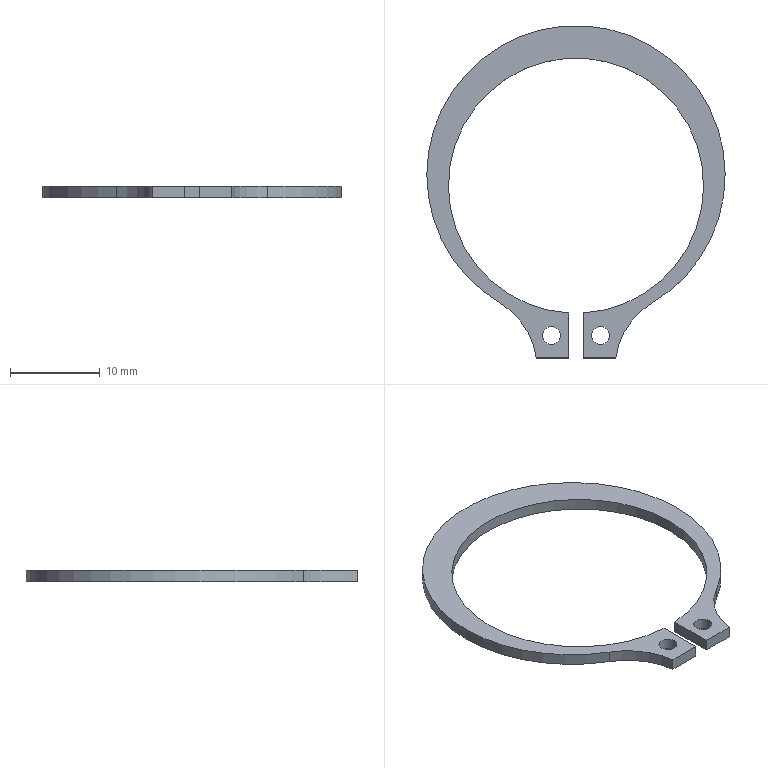Part | SolidWorks | features BaseBody 1 | 1 solid | 15 faces | box 33.15 x 36.925 x 1.3 mm | volume 339.095 mm3 | cylinder 9 | plane 6 | commonest cylinder face diameters 2 x4 16.408 x2 33.15 x2 28.35 x1
STEP:
#1=CARTESIAN_POINT('',(-1.733,-16.65,-1.3));
#2=VERTEX_POINT('',#1);
#3=CARTESIAN_POINT('',(-3.733,-16.65,-1.3));
#4=VERTEX_POINT('',#3);
#5=CARTESIAN_POINT('',(-2.733,-16.65,-1.3));
#6=DIRECTION('',(0.,0.,1.));
#7=DIRECTION('',(-1.,0.,0.));
#8=AXIS2_PLACEMENT_3D('',#5,#6,#7);
#9=CIRCLE('',#8,1.);
#10=EDGE_CURVE('',#2,#4,#9,.T.);
#11=ORIENTED_EDGE('',*,*,#10,.F.);
#12=CARTESIAN_POINT('',(-1.733,-16.65,0.));
#13=VERTEX_POINT('',#12);
#14=CARTESIAN_POINT('',(-1.733,-16.65,0.));
#15=DIRECTION('',(0.,0.,1.));
#16=VECTOR('',#15,1000.);
#17=LINE('',#14,#16);
#18=EDGE_CURVE('',#2,#13,#17,.T.);
#19=ORIENTED_EDGE('',*,*,#18,.T.);
#20=CARTESIAN_POINT('',(-3.733,-16.65,0.));
#21=VERTEX_POINT('',#20);
#22=CARTESIAN_POINT('',(-2.733,-16.65,0.));
#23=DIRECTION('',(0.,0.,-1.));
#24=DIRECTION('',(-1.,0.,0.));
#25=AXIS2_PLACEMENT_3D('',#22,#23,#24);
#26=CIRCLE('',#25,1.);
#27=EDGE_CURVE('',#21,#13,#26,.T.);
#28=ORIENTED_EDGE('',*,*,#27,.F.);
#29=CARTESIAN_POINT('',(-3.733,-16.65,0.));
#30=DIRECTION('',(0.,0.,1.));
#31=VECTOR('',#30,1000.);
#32=LINE('',#29,#31);
#33=EDGE_CURVE('',#4,#21,#32,.T.);
#34=ORIENTED_EDGE('',*,*,#33,.F.);
#35=EDGE_LOOP('',(#11,#19,#28,#34));
#36=FACE_OUTER_BOUND('',#35,.T.);
#37=CARTESIAN_POINT('',(-2.733,-16.65,0.));
#38=DIRECTION('',(0.,0.,1.));
#39=DIRECTION('',(-1.,0.,0.));
#40=AXIS2_PLACEMENT_3D('',#37,#38,#39);
#41=CYLINDRICAL_SURFACE('',#40,1.);
#42=ADVANCED_FACE('',(#36),#41,.F.);
#43=CARTESIAN_POINT('',(3.733,-16.65,-1.3));
#44=VERTEX_POINT('',#43);
#45=CARTESIAN_POINT('',(1.733,-16.65,-1.3));
#46=VERTEX_POINT('',#45);
#47=CARTESIAN_POINT('',(2.733,-16.65,-1.3));
#48=DIRECTION('',(0.,0.,1.));
#49=DIRECTION('',(-1.,0.,0.));
#50=AXIS2_PLACEMENT_3D('',#47,#48,#49);
#51=CIRCLE('',#50,1.);
#52=EDGE_CURVE('',#44,#46,#51,.T.);
#53=ORIENTED_EDGE('',*,*,#52,.F.);
#54=CARTESIAN_POINT('',(3.733,-16.65,0.));
#55=VERTEX_POINT('',#54);
#56=CARTESIAN_POINT('',(3.733,-16.65,0.));
#57=DIRECTION('',(0.,0.,1.));
#58=VECTOR('',#57,1000.);
#59=LINE('',#56,#58);
#60=EDGE_CURVE('',#44,#55,#59,.T.);
#61=ORIENTED_EDGE('',*,*,#60,.T.);
#62=CARTESIAN_POINT('',(1.733,-16.65,0.));
#63=VERTEX_POINT('',#62);
#64=CARTESIAN_POINT('',(2.733,-16.65,0.));
#65=DIRECTION('',(0.,0.,-1.));
#66=DIRECTION('',(-1.,0.,0.));
#67=AXIS2_PLACEMENT_3D('',#64,#65,#66);
#68=CIRCLE('',#67,1.);
#69=EDGE_CURVE('',#63,#55,#68,.T.);
#70=ORIENTED_EDGE('',*,*,#69,.F.);
#71=CARTESIAN_POINT('',(1.733,-16.65,0.));
#72=DIRECTION('',(0.,0.,1.));
#73=VECTOR('',#72,1000.);
#74=LINE('',#71,#73);
#75=EDGE_CURVE('',#46,#63,#74,.T.);
#76=ORIENTED_EDGE('',*,*,#75,.F.);
#77=EDGE_LOOP('',(#53,#61,#70,#76));
#78=FACE_OUTER_BOUND('',#77,.T.);
#79=CARTESIAN_POINT('',(2.733,-16.65,0.));
#80=DIRECTION('',(0.,0.,1.));
#81=DIRECTION('',(-1.,0.,0.));
#82=AXIS2_PLACEMENT_3D('',#79,#80,#81);
#83=CYLINDRICAL_SURFACE('',#82,1.);
#84=ADVANCED_FACE('',(#78),#83,.F.);
#85=CARTESIAN_POINT('',(8.412,-13.082,-1.3));
#86=VERTEX_POINT('',#85);
#87=CARTESIAN_POINT('',(-8.412,15.482,-1.3));
#88=VERTEX_POINT('',#87);
#89=CARTESIAN_POINT('',(0.,1.2,-1.3));
#90=DIRECTION('',(0.,0.,1.));
#91=DIRECTION('',(-0.5075,0.8616,0.));
#92=AXIS2_PLACEMENT_3D('',#89,#90,#91);
#93=CIRCLE('',#92,16.575);
#94=EDGE_CURVE('',#86,#88,#93,.T.);
#95=ORIENTED_EDGE('',*,*,#94,.T.);
#96=CARTESIAN_POINT('',(-8.412,15.482,0.));
#97=VERTEX_POINT('',#96);
#98=CARTESIAN_POINT('',(-8.412,15.482,0.));
#99=DIRECTION('',(0.,0.,1.));
#100=VECTOR('',#99,1000.);
#101=LINE('',#98,#100);
#102=EDGE_CURVE('',#88,#97,#101,.T.);
#103=ORIENTED_EDGE('',*,*,#102,.T.);
#104=CARTESIAN_POINT('',(8.412,-13.082,0.));
#105=VERTEX_POINT('',#104);
#106=CARTESIAN_POINT('',(0.,1.2,0.));
#107=DIRECTION('',(0.,0.,-1.));
#108=DIRECTION('',(-0.5075,0.8616,0.));
#109=AXIS2_PLACEMENT_3D('',#106,#107,#108);
#110=CIRCLE('',#109,16.575);
#111=EDGE_CURVE('',#97,#105,#110,.T.);
#112=ORIENTED_EDGE('',*,*,#111,.T.);
#113=CARTESIAN_POINT('',(8.412,-13.082,0.));
#114=DIRECTION('',(0.,0.,-1.));
#115=VECTOR('',#114,1000.);
#116=LINE('',#113,#115);
#117=EDGE_CURVE('',#105,#86,#116,.T.);
#118=ORIENTED_EDGE('',*,*,#117,.T.);
#119=EDGE_LOOP('',(#95,#103,#112,#118));
#120=FACE_OUTER_BOUND('',#119,.T.);
#121=CARTESIAN_POINT('',(0.,1.2,0.));
#122=DIRECTION('',(0.,0.,1.));
#123=DIRECTION('',(-0.5075,0.8616,0.));
#124=AXIS2_PLACEMENT_3D('',#121,#122,#123);
#125=CYLINDRICAL_SURFACE('',#124,16.575);
#126=ADVANCED_FACE('',(#120),#125,.T.);
#127=CARTESIAN_POINT('',(-0.8333,-19.15,-1.3));
#128=VERTEX_POINT('',#127);
#129=CARTESIAN_POINT('',(-0.8333,-14.15,-1.3));
#130=VERTEX_POINT('',#129);
#131=CARTESIAN_POINT('',(-0.8333,-14.15,-1.3));
#132=DIRECTION('',(0.,1.,0.));
#133=VECTOR('',#132,1000.);
#134=LINE('',#131,#133);
#135=EDGE_CURVE('',#128,#130,#134,.T.);
#136=ORIENTED_EDGE('',*,*,#135,.T.);
#137=CARTESIAN_POINT('',(-0.8333,-14.15,0.));
#138=VERTEX_POINT('',#137);
#139=CARTESIAN_POINT('',(-0.8333,-14.15,0.));
#140=DIRECTION('',(0.,0.,-1.));
#141=VECTOR('',#140,1000.);
#142=LINE('',#139,#141);
#143=EDGE_CURVE('',#138,#130,#142,.T.);
#144=ORIENTED_EDGE('',*,*,#143,.F.);
#145=CARTESIAN_POINT('',(-0.8333,-19.15,0.));
#146=VERTEX_POINT('',#145);
#147=CARTESIAN_POINT('',(-0.8333,-14.15,0.));
#148=DIRECTION('',(0.,-1.,0.));
#149=VECTOR('',#148,1000.);
#150=LINE('',#147,#149);
#151=EDGE_CURVE('',#138,#146,#150,.T.);
#152=ORIENTED_EDGE('',*,*,#151,.T.);
#153=CARTESIAN_POINT('',(-0.8333,-19.15,0.));
#154=DIRECTION('',(0.,0.,-1.));
#155=VECTOR('',#154,1000.);
#156=LINE('',#153,#155);
#157=EDGE_CURVE('',#146,#128,#156,.T.);
#158=ORIENTED_EDGE('',*,*,#157,.T.);
#159=EDGE_LOOP('',(#136,#144,#152,#158));
#160=FACE_OUTER_BOUND('',#159,.T.);
#161=CARTESIAN_POINT('',(-0.8333,-19.15,0.));
#162=DIRECTION('',(1.,0.,0.));
#163=DIRECTION('',(0.,1.,0.));
#164=AXIS2_PLACEMENT_3D('',#161,#162,#163);
#165=PLANE('',#164);
#166=ADVANCED_FACE('',(#160),#165,.T.);
#167=CARTESIAN_POINT('',(0.8333,-14.15,-1.3));
#168=VERTEX_POINT('',#167);
#169=CARTESIAN_POINT('',(0.,0.,-1.3));
#170=DIRECTION('',(0.,0.,-1.));
#171=DIRECTION('',(0.05879,-0.9983,0.));
#172=AXIS2_PLACEMENT_3D('',#169,#170,#171);
#173=CIRCLE('',#172,14.175);
#174=EDGE_CURVE('',#130,#168,#173,.T.);
#175=ORIENTED_EDGE('',*,*,#174,.T.);
#176=CARTESIAN_POINT('',(0.8333,-14.15,0.));
#177=VERTEX_POINT('',#176);
#178=CARTESIAN_POINT('',(0.8333,-14.15,0.));
#179=DIRECTION('',(0.,0.,-1.));
#180=VECTOR('',#179,1000.);
#181=LINE('',#178,#180);
#182=EDGE_CURVE('',#177,#168,#181,.T.);
#183=ORIENTED_EDGE('',*,*,#182,.F.);
#184=CARTESIAN_POINT('',(0.,0.,0.));
#185=DIRECTION('',(0.,0.,1.));
#186=DIRECTION('',(0.05879,-0.9983,0.));
#187=AXIS2_PLACEMENT_3D('',#184,#185,#186);
#188=CIRCLE('',#187,14.175);
#189=EDGE_CURVE('',#177,#138,#188,.T.);
#190=ORIENTED_EDGE('',*,*,#189,.T.);
#191=ORIENTED_EDGE('',*,*,#143,.T.);
#192=EDGE_LOOP('',(#175,#183,#190,#191));
#193=FACE_OUTER_BOUND('',#192,.T.);
#194=CARTESIAN_POINT('',(0.,0.,0.));
#195=DIRECTION('',(0.,0.,1.));
#196=DIRECTION('',(0.05879,-0.9983,0.));
#197=AXIS2_PLACEMENT_3D('',#194,#195,#196);
#198=CYLINDRICAL_SURFACE('',#197,14.175);
#199=ADVANCED_FACE('',(#193),#198,.F.);
#200=CARTESIAN_POINT('',(0.8333,-19.15,-1.3));
#201=VERTEX_POINT('',#200);
#202=CARTESIAN_POINT('',(0.8333,-19.15,-1.3));
#203=DIRECTION('',(0.,-1.,0.));
#204=VECTOR('',#203,1000.);
#205=LINE('',#202,#204);
#206=EDGE_CURVE('',#168,#201,#205,.T.);
#207=ORIENTED_EDGE('',*,*,#206,.T.);
#208=CARTESIAN_POINT('',(0.8333,-19.15,0.));
#209=VERTEX_POINT('',#208);
#210=CARTESIAN_POINT('',(0.8333,-19.15,0.));
#211=DIRECTION('',(0.,0.,-1.));
#212=VECTOR('',#211,1000.);
#213=LINE('',#210,#212);
#214=EDGE_CURVE('',#209,#201,#213,.T.);
#215=ORIENTED_EDGE('',*,*,#214,.F.);
#216=CARTESIAN_POINT('',(0.8333,-19.15,0.));
#217=DIRECTION('',(0.,1.,0.));
#218=VECTOR('',#217,1000.);
#219=LINE('',#216,#218);
#220=EDGE_CURVE('',#209,#177,#219,.T.);
#221=ORIENTED_EDGE('',*,*,#220,.T.);
#222=ORIENTED_EDGE('',*,*,#182,.T.);
#223=EDGE_LOOP('',(#207,#215,#221,#222));
#224=FACE_OUTER_BOUND('',#223,.T.);
#225=CARTESIAN_POINT('',(0.8333,-14.15,0.));
#226=DIRECTION('',(-1.,0.,0.));
#227=DIRECTION('',(0.,0.,1.));
#228=AXIS2_PLACEMENT_3D('',#225,#226,#227);
#229=PLANE('',#228);
#230=ADVANCED_FACE('',(#224),#229,.T.);
#231=CARTESIAN_POINT('',(4.433,-19.15,-1.3));
#232=VERTEX_POINT('',#231);
#233=CARTESIAN_POINT('',(4.433,-19.15,-1.3));
#234=DIRECTION('',(1.,0.,0.));
#235=VECTOR('',#234,1000.);
#236=LINE('',#233,#235);
#237=EDGE_CURVE('',#201,#232,#236,.T.);
#238=ORIENTED_EDGE('',*,*,#237,.T.);
#239=CARTESIAN_POINT('',(4.433,-19.15,0.));
#240=VERTEX_POINT('',#239);
#241=CARTESIAN_POINT('',(4.433,-19.15,0.));
#242=DIRECTION('',(0.,0.,-1.));
#243=VECTOR('',#242,1000.);
#244=LINE('',#241,#243);
#245=EDGE_CURVE('',#240,#232,#244,.T.);
#246=ORIENTED_EDGE('',*,*,#245,.F.);
#247=CARTESIAN_POINT('',(4.433,-19.15,0.));
#248=DIRECTION('',(-1.,0.,0.));
#249=VECTOR('',#248,1000.);
#250=LINE('',#247,#249);
#251=EDGE_CURVE('',#240,#209,#250,.T.);
#252=ORIENTED_EDGE('',*,*,#251,.T.);
#253=ORIENTED_EDGE('',*,*,#214,.T.);
#254=EDGE_LOOP('',(#238,#246,#252,#253));
#255=FACE_OUTER_BOUND('',#254,.T.);
#256=CARTESIAN_POINT('',(0.8333,-19.15,0.));
#257=DIRECTION('',(0.,-1.,0.));
#258=DIRECTION('',(-1.,0.,0.));
#259=AXIS2_PLACEMENT_3D('',#256,#257,#258);
#260=PLANE('',#259);
#261=ADVANCED_FACE('',(#255),#260,.T.);
#262=CARTESIAN_POINT('',(12.576,-20.15,-1.3));
#263=DIRECTION('',(0.,0.,-1.));
#264=DIRECTION('',(-0.5075,0.8616,0.));
#265=AXIS2_PLACEMENT_3D('',#262,#263,#264);
#266=CIRCLE('',#265,8.204);
#267=EDGE_CURVE('',#232,#86,#266,.T.);
#268=ORIENTED_EDGE('',*,*,#267,.T.);
#269=ORIENTED_EDGE('',*,*,#117,.F.);
#270=CARTESIAN_POINT('',(12.576,-20.15,0.));
#271=DIRECTION('',(0.,0.,1.));
#272=DIRECTION('',(-0.5075,0.8616,0.));
#273=AXIS2_PLACEMENT_3D('',#270,#271,#272);
#274=CIRCLE('',#273,8.204);
#275=EDGE_CURVE('',#105,#240,#274,.T.);
#276=ORIENTED_EDGE('',*,*,#275,.T.);
#277=ORIENTED_EDGE('',*,*,#245,.T.);
#278=EDGE_LOOP('',(#268,#269,#276,#277));
#279=FACE_OUTER_BOUND('',#278,.T.);
#280=CARTESIAN_POINT('',(12.576,-20.15,0.));
#281=DIRECTION('',(0.,0.,1.));
#282=DIRECTION('',(-0.5075,0.8616,0.));
#283=AXIS2_PLACEMENT_3D('',#280,#281,#282);
#284=CYLINDRICAL_SURFACE('',#283,8.204);
#285=ADVANCED_FACE('',(#279),#284,.F.);
#286=CARTESIAN_POINT('',(-8.412,-13.082,-1.3));
#287=VERTEX_POINT('',#286);
#288=CARTESIAN_POINT('',(-4.433,-19.15,-1.3));
#289=VERTEX_POINT('',#288);
#290=CARTESIAN_POINT('',(-12.576,-20.15,-1.3));
#291=DIRECTION('',(0.,0.,-1.));
#292=DIRECTION('',(0.9925,0.1219,0.));
#293=AXIS2_PLACEMENT_3D('',#290,#291,#292);
#294=CIRCLE('',#293,8.204);
#295=EDGE_CURVE('',#287,#289,#294,.T.);
#296=ORIENTED_EDGE('',*,*,#295,.T.);
#297=CARTESIAN_POINT('',(-4.433,-19.15,0.));
#298=VERTEX_POINT('',#297);
#299=CARTESIAN_POINT('',(-4.433,-19.15,0.));
#300=DIRECTION('',(0.,0.,-1.));
#301=VECTOR('',#300,1000.);
#302=LINE('',#299,#301);
#303=EDGE_CURVE('',#298,#289,#302,.T.);
#304=ORIENTED_EDGE('',*,*,#303,.F.);
#305=CARTESIAN_POINT('',(-8.412,-13.082,0.));
#306=VERTEX_POINT('',#305);
#307=CARTESIAN_POINT('',(-12.576,-20.15,0.));
#308=DIRECTION('',(0.,0.,1.));
#309=DIRECTION('',(0.9925,0.1219,0.));
#310=AXIS2_PLACEMENT_3D('',#307,#308,#309);
#311=CIRCLE('',#310,8.204);
#312=EDGE_CURVE('',#298,#306,#311,.T.);
#313=ORIENTED_EDGE('',*,*,#312,.T.);
#314=CARTESIAN_POINT('',(-8.412,-13.082,0.));
#315=DIRECTION('',(0.,0.,-1.));
#316=VECTOR('',#315,1000.);
#317=LINE('',#314,#316);
#318=EDGE_CURVE('',#306,#287,#317,.T.);
#319=ORIENTED_EDGE('',*,*,#318,.T.);
#320=EDGE_LOOP('',(#296,#304,#313,#319));
#321=FACE_OUTER_BOUND('',#320,.T.);
#322=CARTESIAN_POINT('',(-12.576,-20.15,0.));
#323=DIRECTION('',(0.,0.,1.));
#324=DIRECTION('',(0.9925,0.1219,0.));
#325=AXIS2_PLACEMENT_3D('',#322,#323,#324);
#326=CYLINDRICAL_SURFACE('',#325,8.204);
#327=ADVANCED_FACE('',(#321),#326,.F.);
#328=CARTESIAN_POINT('',(-0.8333,-19.15,-1.3));
#329=DIRECTION('',(1.,0.,0.));
#330=VECTOR('',#329,1000.);
#331=LINE('',#328,#330);
#332=EDGE_CURVE('',#289,#128,#331,.T.);
#333=ORIENTED_EDGE('',*,*,#332,.T.);
#334=ORIENTED_EDGE('',*,*,#157,.F.);
#335=CARTESIAN_POINT('',(-0.8333,-19.15,0.));
#336=DIRECTION('',(-1.,0.,0.));
#337=VECTOR('',#336,1000.);
#338=LINE('',#335,#337);
#339=EDGE_CURVE('',#146,#298,#338,.T.);
#340=ORIENTED_EDGE('',*,*,#339,.T.);
#341=ORIENTED_EDGE('',*,*,#303,.T.);
#342=EDGE_LOOP('',(#333,#334,#340,#341));
#343=FACE_OUTER_BOUND('',#342,.T.);
#344=CARTESIAN_POINT('',(-4.433,-19.15,0.));
#345=DIRECTION('',(0.,-1.,0.));
#346=DIRECTION('',(0.,0.,-1.));
#347=AXIS2_PLACEMENT_3D('',#344,#345,#346);
#348=PLANE('',#347);
#349=ADVANCED_FACE('',(#343),#348,.T.);
#350=ORIENTED_EDGE('',*,*,#27,.T.);
#351=CARTESIAN_POINT('',(-2.733,-16.65,0.));
#352=DIRECTION('',(0.,0.,-1.));
#353=DIRECTION('',(-1.,0.,0.));
#354=AXIS2_PLACEMENT_3D('',#351,#352,#353);
#355=CIRCLE('',#354,1.);
#356=EDGE_CURVE('',#13,#21,#355,.T.);
#357=ORIENTED_EDGE('',*,*,#356,.T.);
#358=EDGE_LOOP('',(#350,#357));
#359=FACE_BOUND('',#358,.T.);
#360=ORIENTED_EDGE('',*,*,#69,.T.);
#361=CARTESIAN_POINT('',(2.733,-16.65,0.));
#362=DIRECTION('',(0.,0.,-1.));
#363=DIRECTION('',(-1.,0.,0.));
#364=AXIS2_PLACEMENT_3D('',#361,#362,#363);
#365=CIRCLE('',#364,1.);
#366=EDGE_CURVE('',#55,#63,#365,.T.);
#367=ORIENTED_EDGE('',*,*,#366,.T.);
#368=EDGE_LOOP('',(#360,#367));
#369=FACE_BOUND('',#368,.T.);
#370=ORIENTED_EDGE('',*,*,#339,.F.);
#371=ORIENTED_EDGE('',*,*,#151,.F.);
#372=ORIENTED_EDGE('',*,*,#189,.F.);
#373=ORIENTED_EDGE('',*,*,#220,.F.);
#374=ORIENTED_EDGE('',*,*,#251,.F.);
#375=ORIENTED_EDGE('',*,*,#275,.F.);
#376=ORIENTED_EDGE('',*,*,#111,.F.);
#377=CARTESIAN_POINT('',(0.,1.2,0.));
#378=DIRECTION('',(0.,0.,-1.));
#379=DIRECTION('',(-0.5075,0.8616,0.));
#380=AXIS2_PLACEMENT_3D('',#377,#378,#379);
#381=CIRCLE('',#380,16.575);
#382=EDGE_CURVE('',#306,#97,#381,.T.);
#383=ORIENTED_EDGE('',*,*,#382,.F.);
#384=ORIENTED_EDGE('',*,*,#312,.F.);
#385=EDGE_LOOP('',(#370,#371,#372,#373,#374,#375,#376,#383,#384));
#386=FACE_OUTER_BOUND('',#385,.T.);
#387=CARTESIAN_POINT('',(0.,-1.916,0.));
#388=DIRECTION('',(0.,0.,1.));
#389=DIRECTION('',(1.,0.,0.));
#390=AXIS2_PLACEMENT_3D('',#387,#388,#389);
#391=PLANE('',#390);
#392=ADVANCED_FACE('',(#359,#369,#386),#391,.T.);
#393=CARTESIAN_POINT('',(-2.733,-16.65,-1.3));
#394=DIRECTION('',(0.,0.,1.));
#395=DIRECTION('',(-1.,0.,0.));
#396=AXIS2_PLACEMENT_3D('',#393,#394,#395);
#397=CIRCLE('',#396,1.);
#398=EDGE_CURVE('',#4,#2,#397,.T.);
#399=ORIENTED_EDGE('',*,*,#398,.T.);
#400=ORIENTED_EDGE('',*,*,#10,.T.);
#401=EDGE_LOOP('',(#399,#400));
#402=FACE_BOUND('',#401,.T.);
#403=CARTESIAN_POINT('',(2.733,-16.65,-1.3));
#404=DIRECTION('',(0.,0.,1.));
#405=DIRECTION('',(-1.,0.,0.));
#406=AXIS2_PLACEMENT_3D('',#403,#404,#405);
#407=CIRCLE('',#406,1.);
#408=EDGE_CURVE('',#46,#44,#407,.T.);
#409=ORIENTED_EDGE('',*,*,#408,.T.);
#410=ORIENTED_EDGE('',*,*,#52,.T.);
#411=EDGE_LOOP('',(#409,#410));
#412=FACE_BOUND('',#411,.T.);
#413=ORIENTED_EDGE('',*,*,#135,.F.);
#414=ORIENTED_EDGE('',*,*,#332,.F.);
#415=ORIENTED_EDGE('',*,*,#295,.F.);
#416=CARTESIAN_POINT('',(0.,1.2,-1.3));
#417=DIRECTION('',(0.,0.,1.));
#418=DIRECTION('',(-0.5075,0.8616,0.));
#419=AXIS2_PLACEMENT_3D('',#416,#417,#418);
#420=CIRCLE('',#419,16.575);
#421=EDGE_CURVE('',#88,#287,#420,.T.);
#422=ORIENTED_EDGE('',*,*,#421,.F.);
#423=ORIENTED_EDGE('',*,*,#94,.F.);
#424=ORIENTED_EDGE('',*,*,#267,.F.);
#425=ORIENTED_EDGE('',*,*,#237,.F.);
#426=ORIENTED_EDGE('',*,*,#206,.F.);
#427=ORIENTED_EDGE('',*,*,#174,.F.);
#428=EDGE_LOOP('',(#413,#414,#415,#422,#423,#424,#425,#426,#427));
#429=FACE_OUTER_BOUND('',#428,.T.);
#430=CARTESIAN_POINT('',(0.,-1.916,-1.3));
#431=DIRECTION('',(0.,0.,1.));
#432=DIRECTION('',(1.,0.,0.));
#433=AXIS2_PLACEMENT_3D('',#430,#431,#432);
#434=PLANE('',#433);
#435=ADVANCED_FACE('',(#402,#412,#429),#434,.F.);
#436=ORIENTED_EDGE('',*,*,#102,.F.);
#437=ORIENTED_EDGE('',*,*,#421,.T.);
#438=ORIENTED_EDGE('',*,*,#318,.F.);
#439=ORIENTED_EDGE('',*,*,#382,.T.);
#440=EDGE_LOOP('',(#436,#437,#438,#439));
#441=FACE_OUTER_BOUND('',#440,.T.);
#442=CARTESIAN_POINT('',(0.,1.2,0.));
#443=DIRECTION('',(0.,0.,1.));
#444=DIRECTION('',(-0.5075,0.8616,0.));
#445=AXIS2_PLACEMENT_3D('',#442,#443,#444);
#446=CYLINDRICAL_SURFACE('',#445,16.575);
#447=ADVANCED_FACE('',(#441),#446,.T.);
#448=ORIENTED_EDGE('',*,*,#60,.F.);
#449=ORIENTED_EDGE('',*,*,#408,.F.);
#450=ORIENTED_EDGE('',*,*,#75,.T.);
#451=ORIENTED_EDGE('',*,*,#366,.F.);
#452=EDGE_LOOP('',(#448,#449,#450,#451));
#453=FACE_OUTER_BOUND('',#452,.T.);
#454=CARTESIAN_POINT('',(2.733,-16.65,0.));
#455=DIRECTION('',(0.,0.,1.));
#456=DIRECTION('',(-1.,0.,0.));
#457=AXIS2_PLACEMENT_3D('',#454,#455,#456);
#458=CYLINDRICAL_SURFACE('',#457,1.);
#459=ADVANCED_FACE('',(#453),#458,.F.);
#460=ORIENTED_EDGE('',*,*,#18,.F.);
#461=ORIENTED_EDGE('',*,*,#398,.F.);
#462=ORIENTED_EDGE('',*,*,#33,.T.);
#463=ORIENTED_EDGE('',*,*,#356,.F.);
#464=EDGE_LOOP('',(#460,#461,#462,#463));
#465=FACE_OUTER_BOUND('',#464,.T.);
#466=CARTESIAN_POINT('',(-2.733,-16.65,0.));
#467=DIRECTION('',(0.,0.,1.));
#468=DIRECTION('',(-1.,0.,0.));
#469=AXIS2_PLACEMENT_3D('',#466,#467,#468);
#470=CYLINDRICAL_SURFACE('',#469,1.);
#471=ADVANCED_FACE('',(#465),#470,.F.);
#472=CLOSED_SHELL('',(#42,#84,#126,#166,#199,#230,#261,#285,#327,#349,#392,#435,#447,#459,#471));
#473=MANIFOLD_SOLID_BREP('',#472);
#474=CARTESIAN_POINT('',(0.,0.,0.));
#475=DIRECTION('',(0.,0.,1.));
#476=DIRECTION('',(1.,0.,0.));
#477=AXIS2_PLACEMENT_3D('',#474,#475,#476);
#478=(LENGTH_UNIT()NAMED_UNIT(*)SI_UNIT(.MILLI.,.METRE.));
#479=UNCERTAINTY_MEASURE_WITH_UNIT(LENGTH_MEASURE(0.00001),#478,'','');
#480=(NAMED_UNIT(*)PLANE_ANGLE_UNIT()SI_UNIT($,.RADIAN.));
#481=(NAMED_UNIT(*)SI_UNIT($,.STERADIAN.)SOLID_ANGLE_UNIT());
#482=(GEOMETRIC_REPRESENTATION_CONTEXT(3)GLOBAL_UNCERTAINTY_ASSIGNED_CONTEXT((#479))GLOBAL_UNIT_ASSIGNED_CONTEXT((#478,#480,#481))REPRESENTATION_CONTEXT('',''));
#483=ADVANCED_BREP_SHAPE_REPRESENTATION('',(#473,#477),#482);